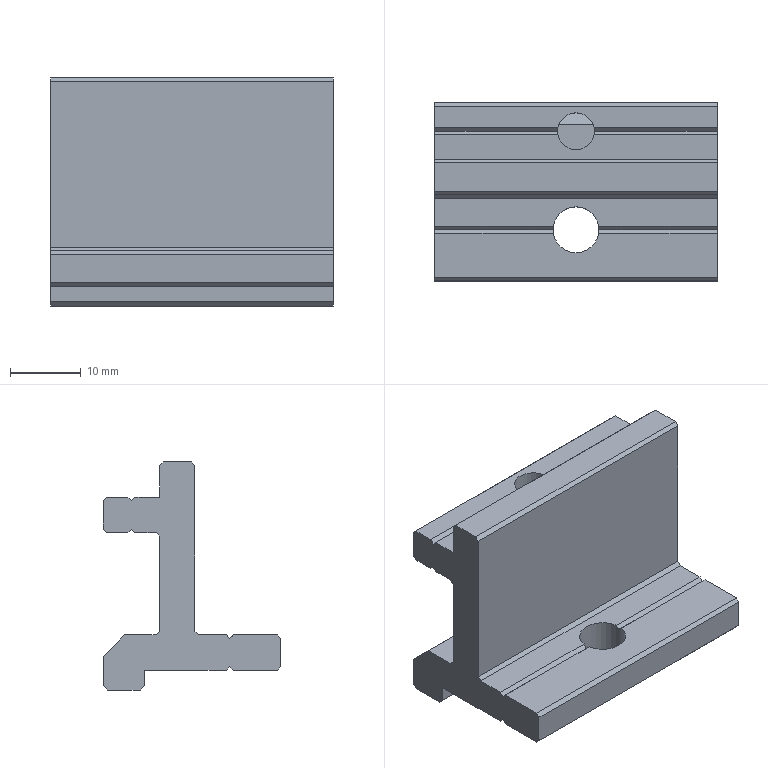Part | NX | features DATUM_CSYS 3, EXTRUDE 3, SKETCH 2 | 1 solid | 50 faces | box 40 x 25.175 x 32.3 mm | volume 11675 mm3 | plane 48 | cylinder 2 | commonest cylinder face diameters 5.2 x1 6.5 x1